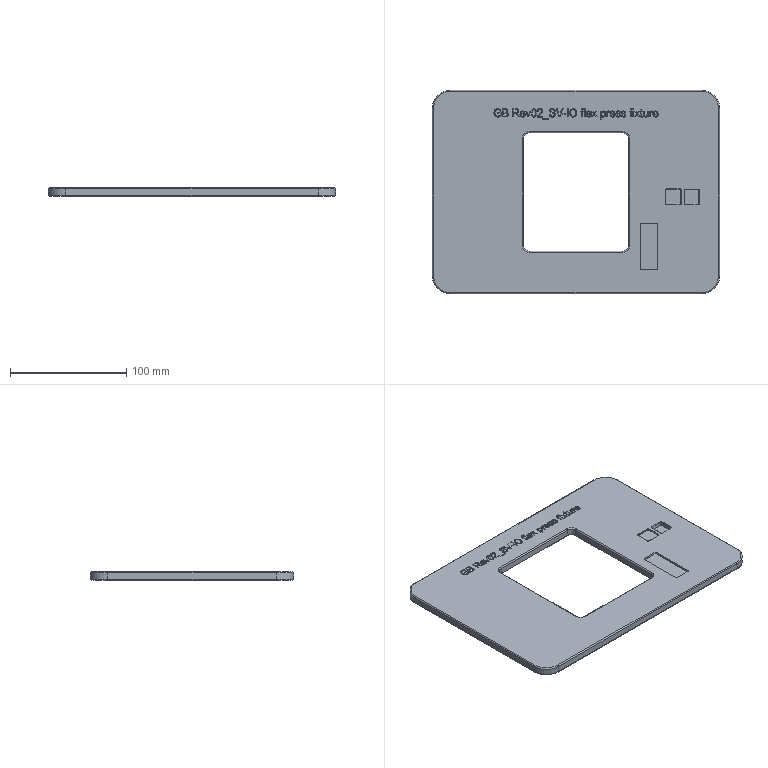Part | 1 solid | 345 faces | box 247.208 x 175.016 x 7.2 mm | volume 237023 mm3 | plane 218 | spline 57 | cylinder 46 | torus 16 | cone 8 | commonest cylinder face diameters 2 x20 1.2 x8 10 x4 22 x4 30 x4 123.527 x2